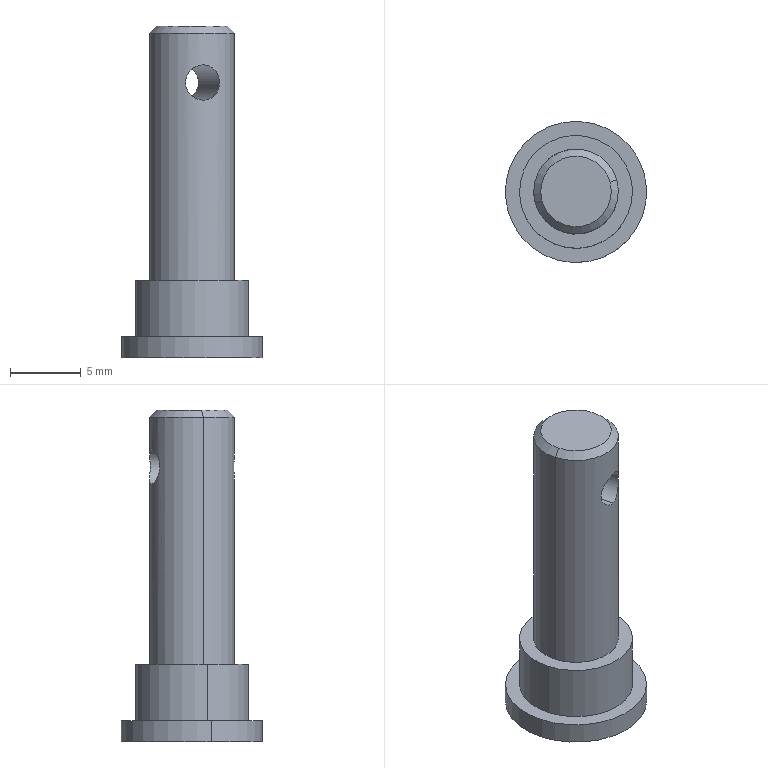Part | SolidWorks | features BaseBody 1 | 1 solid | 14 faces | box 10 x 10 x 23.5 mm | volume 796.786 mm3 | cylinder 8 | plane 4 | cone 2 | commonest cylinder face diameters 2.5 x2 6 x2 8 x2 10 x2
STEP:
#1=CARTESIAN_POINT('',(437.007,50.123,99.45));
#2=VERTEX_POINT('',#1);
#3=CARTESIAN_POINT('',(437.007,50.123,101.95));
#4=VERTEX_POINT('',#3);
#5=CARTESIAN_POINT('',(437.007,50.123,99.45));
#6=CARTESIAN_POINT('',(437.165,50.167,99.45));
#7=CARTESIAN_POINT('',(437.329,50.199,99.483));
#8=CARTESIAN_POINT('',(437.633,50.233,99.61));
#9=CARTESIAN_POINT('',(437.774,50.237,99.702));
#10=CARTESIAN_POINT('',(437.954,50.233,99.874));
#11=CARTESIAN_POINT('',(438.008,50.23,99.937));
#12=CARTESIAN_POINT('',(438.104,50.223,100.071));
#13=CARTESIAN_POINT('',(438.146,50.218,100.144));
#14=CARTESIAN_POINT('',(438.214,50.21,100.294));
#15=CARTESIAN_POINT('',(438.239,50.206,100.372));
#16=CARTESIAN_POINT('',(438.275,50.201,100.533));
#17=CARTESIAN_POINT('',(438.284,50.2,100.617));
#18=CARTESIAN_POINT('',(438.284,50.2,100.864));
#19=CARTESIAN_POINT('',(438.247,50.206,101.03));
#20=CARTESIAN_POINT('',(438.112,50.222,101.332));
#21=CARTESIAN_POINT('',(438.014,50.232,101.469));
#22=CARTESIAN_POINT('',(437.774,50.237,101.698));
#23=CARTESIAN_POINT('',(437.635,50.234,101.79));
#24=CARTESIAN_POINT('',(437.328,50.199,101.917));
#25=CARTESIAN_POINT('',(437.168,50.168,101.95));
#26=CARTESIAN_POINT('',(437.007,50.123,101.95));
#27=B_SPLINE_CURVE_WITH_KNOTS('',3,(#5,#6,#7,#8,#9,#10,#11,#12,#13,#14,#15,#16,#17,#18,#19,#20,#21,#22,#23,#24,#25,#26),.UNSPECIFIED.,.F.,.F.,(4,2,2,2,2,2,2,2,2,2,4),(0.003954,0.004448,0.004941,0.005188,0.005435,0.005682,0.005929,0.006423,0.006917,0.00741,0.007904),.UNSPECIFIED.);
#28=EDGE_CURVE('',#2,#4,#27,.T.);
#29=ORIENTED_EDGE('',*,*,#28,.F.);
#30=CARTESIAN_POINT('',(438.637,44.348,99.45));
#31=VERTEX_POINT('',#30);
#32=CARTESIAN_POINT('',(436.463,52.047,99.45));
#33=DIRECTION('',(0.2716,-0.9624,0.));
#34=VECTOR('',#33,1000.);
#35=LINE('',#32,#34);
#36=EDGE_CURVE('',#2,#31,#35,.T.);
#37=ORIENTED_EDGE('',*,*,#36,.T.);
#38=CARTESIAN_POINT('',(438.637,44.348,101.95));
#39=VERTEX_POINT('',#38);
#40=CARTESIAN_POINT('',(438.637,44.348,101.95));
#41=CARTESIAN_POINT('',(438.717,44.371,101.95));
#42=CARTESIAN_POINT('',(438.795,44.397,101.942));
#43=CARTESIAN_POINT('',(438.946,44.453,101.909));
#44=CARTESIAN_POINT('',(439.021,44.484,101.885));
#45=CARTESIAN_POINT('',(439.229,44.581,101.79));
#46=CARTESIAN_POINT('',(439.352,44.652,101.697));
#47=CARTESIAN_POINT('',(439.552,44.782,101.469));
#48=CARTESIAN_POINT('',(439.631,44.841,101.332));
#49=CARTESIAN_POINT('',(439.737,44.926,101.032));
#50=CARTESIAN_POINT('',(439.765,44.95,100.866));
#51=CARTESIAN_POINT('',(439.765,44.95,100.618));
#52=CARTESIAN_POINT('',(439.758,44.944,100.534));
#53=CARTESIAN_POINT('',(439.731,44.922,100.373));
#54=CARTESIAN_POINT('',(439.711,44.905,100.294));
#55=CARTESIAN_POINT('',(439.63,44.841,100.066));
#56=CARTESIAN_POINT('',(439.551,44.781,99.93));
#57=CARTESIAN_POINT('',(439.35,44.651,99.702));
#58=CARTESIAN_POINT('',(439.227,44.581,99.609));
#59=CARTESIAN_POINT('',(438.951,44.452,99.484));
#60=CARTESIAN_POINT('',(438.795,44.393,99.45));
#61=CARTESIAN_POINT('',(438.637,44.348,99.45));
#62=B_SPLINE_CURVE_WITH_KNOTS('',3,(#40,#41,#42,#43,#44,#45,#46,#47,#48,#49,#50,#51,#52,#53,#54,#55,#56,#57,#58,#59,#60,#61),.UNSPECIFIED.,.F.,.F.,(4,2,2,2,2,2,2,2,2,2,4),(0.,0.0002471,0.0004942,0.0009884,0.001483,0.001977,0.002224,0.002471,0.002965,0.003459,0.003954),.UNSPECIFIED.);
#63=EDGE_CURVE('',#39,#31,#62,.T.);
#64=ORIENTED_EDGE('',*,*,#63,.F.);
#65=CARTESIAN_POINT('',(436.463,52.047,101.95));
#66=DIRECTION('',(0.2716,-0.9624,0.));
#67=VECTOR('',#66,1000.);
#68=LINE('',#65,#67);
#69=EDGE_CURVE('',#4,#39,#68,.T.);
#70=ORIENTED_EDGE('',*,*,#69,.F.);
#71=EDGE_LOOP('',(#29,#37,#64,#70));
#72=FACE_OUTER_BOUND('',#71,.T.);
#73=CARTESIAN_POINT('',(436.463,52.047,100.7));
#74=DIRECTION('',(0.2716,-0.9624,0.));
#75=DIRECTION('',(0.,0.,1.));
#76=AXIS2_PLACEMENT_3D('',#73,#74,#75);
#77=CYLINDRICAL_SURFACE('',#76,1.25);
#78=ADVANCED_FACE('',(#72),#77,.F.);
#79=CARTESIAN_POINT('',(435.416,46.556,104.7));
#80=VERTEX_POINT('',#79);
#81=CARTESIAN_POINT('',(440.228,47.915,104.7));
#82=VERTEX_POINT('',#81);
#83=CARTESIAN_POINT('',(437.822,47.235,104.7));
#84=DIRECTION('',(0.,0.,1.));
#85=DIRECTION('',(-0.9624,-0.2716,0.));
#86=AXIS2_PLACEMENT_3D('',#83,#84,#85);
#87=CIRCLE('',#86,2.5);
#88=EDGE_CURVE('',#80,#82,#87,.T.);
#89=ORIENTED_EDGE('',*,*,#88,.F.);
#90=CARTESIAN_POINT('',(434.934,46.421,104.2));
#91=VERTEX_POINT('',#90);
#92=CARTESIAN_POINT('',(435.416,46.556,104.7));
#93=DIRECTION('',(-0.6805,-0.1921,-0.7071));
#94=VECTOR('',#93,1000.);
#95=LINE('',#92,#94);
#96=EDGE_CURVE('',#80,#91,#95,.T.);
#97=ORIENTED_EDGE('',*,*,#96,.T.);
#98=CARTESIAN_POINT('',(440.709,48.05,104.2));
#99=VERTEX_POINT('',#98);
#100=CARTESIAN_POINT('',(437.822,47.235,104.2));
#101=DIRECTION('',(0.,0.,-1.));
#102=DIRECTION('',(-0.9624,-0.2716,0.));
#103=AXIS2_PLACEMENT_3D('',#100,#101,#102);
#104=CIRCLE('',#103,3.);
#105=EDGE_CURVE('',#99,#91,#104,.T.);
#106=ORIENTED_EDGE('',*,*,#105,.F.);
#107=CARTESIAN_POINT('',(440.228,47.915,104.7));
#108=DIRECTION('',(0.6805,0.1921,-0.7071));
#109=VECTOR('',#108,1000.);
#110=LINE('',#107,#109);
#111=EDGE_CURVE('',#82,#99,#110,.T.);
#112=ORIENTED_EDGE('',*,*,#111,.F.);
#113=EDGE_LOOP('',(#89,#97,#106,#112));
#114=FACE_OUTER_BOUND('',#113,.T.);
#115=CARTESIAN_POINT('',(437.822,47.235,104.7));
#116=DIRECTION('',(0.,0.,-1.));
#117=DIRECTION('',(0.9624,0.2716,0.));
#118=AXIS2_PLACEMENT_3D('',#115,#116,#117);
#119=CONICAL_SURFACE('',#118,2.5,0.7854);
#120=ADVANCED_FACE('',(#114),#119,.T.);
#121=ORIENTED_EDGE('',*,*,#63,.T.);
#122=CARTESIAN_POINT('',(438.637,44.348,99.45));
#123=CARTESIAN_POINT('',(438.478,44.304,99.45));
#124=CARTESIAN_POINT('',(438.315,44.272,99.483));
#125=CARTESIAN_POINT('',(438.01,44.237,99.61));
#126=CARTESIAN_POINT('',(437.869,44.233,99.702));
#127=CARTESIAN_POINT('',(437.689,44.238,99.874));
#128=CARTESIAN_POINT('',(437.635,44.241,99.937));
#129=CARTESIAN_POINT('',(437.539,44.248,100.071));
#130=CARTESIAN_POINT('',(437.497,44.253,100.144));
#131=CARTESIAN_POINT('',(437.43,44.261,100.294));
#132=CARTESIAN_POINT('',(437.404,44.265,100.372));
#133=CARTESIAN_POINT('',(437.369,44.27,100.533));
#134=CARTESIAN_POINT('',(437.359,44.271,100.617));
#135=CARTESIAN_POINT('',(437.359,44.271,100.864));
#136=CARTESIAN_POINT('',(437.396,44.265,101.03));
#137=CARTESIAN_POINT('',(437.531,44.249,101.332));
#138=CARTESIAN_POINT('',(437.629,44.239,101.469));
#139=CARTESIAN_POINT('',(437.869,44.233,101.698));
#140=CARTESIAN_POINT('',(438.009,44.237,101.79));
#141=CARTESIAN_POINT('',(438.315,44.272,101.917));
#142=CARTESIAN_POINT('',(438.476,44.303,101.95));
#143=CARTESIAN_POINT('',(438.637,44.348,101.95));
#144=B_SPLINE_CURVE_WITH_KNOTS('',3,(#122,#123,#124,#125,#126,#127,#128,#129,#130,#131,#132,#133,#134,#135,#136,#137,#138,#139,#140,#141,#142,#143),.UNSPECIFIED.,.F.,.F.,(4,2,2,2,2,2,2,2,2,2,4),(0.003954,0.004448,0.004941,0.005188,0.005435,0.005682,0.005929,0.006423,0.006917,0.00741,0.007904),.UNSPECIFIED.);
#145=EDGE_CURVE('',#31,#39,#144,.T.);
#146=ORIENTED_EDGE('',*,*,#145,.T.);
#147=EDGE_LOOP('',(#121,#146));
#148=FACE_BOUND('',#147,.T.);
#149=ORIENTED_EDGE('',*,*,#105,.T.);
#150=CARTESIAN_POINT('',(434.934,46.421,86.7));
#151=VERTEX_POINT('',#150);
#152=CARTESIAN_POINT('',(434.934,46.421,104.7));
#153=DIRECTION('',(0.,0.,-1.));
#154=VECTOR('',#153,1000.);
#155=LINE('',#152,#154);
#156=EDGE_CURVE('',#91,#151,#155,.T.);
#157=ORIENTED_EDGE('',*,*,#156,.T.);
#158=CARTESIAN_POINT('',(440.709,48.05,86.7));
#159=VERTEX_POINT('',#158);
#160=CARTESIAN_POINT('',(437.822,47.235,86.7));
#161=DIRECTION('',(0.,0.,1.));
#162=DIRECTION('',(-0.9624,-0.2716,0.));
#163=AXIS2_PLACEMENT_3D('',#160,#161,#162);
#164=CIRCLE('',#163,3.);
#165=EDGE_CURVE('',#151,#159,#164,.T.);
#166=ORIENTED_EDGE('',*,*,#165,.T.);
#167=CARTESIAN_POINT('',(440.709,48.05,104.7));
#168=DIRECTION('',(0.,0.,-1.));
#169=VECTOR('',#168,1000.);
#170=LINE('',#167,#169);
#171=EDGE_CURVE('',#99,#159,#170,.T.);
#172=ORIENTED_EDGE('',*,*,#171,.F.);
#173=EDGE_LOOP('',(#149,#157,#166,#172));
#174=FACE_OUTER_BOUND('',#173,.T.);
#175=CARTESIAN_POINT('',(437.822,47.235,104.7));
#176=DIRECTION('',(0.,0.,-1.));
#177=DIRECTION('',(0.9624,0.2716,0.));
#178=AXIS2_PLACEMENT_3D('',#175,#176,#177);
#179=CYLINDRICAL_SURFACE('',#178,3.);
#180=ADVANCED_FACE('',(#148,#174),#179,.T.);
#181=CARTESIAN_POINT('',(433.972,46.149,86.7));
#182=VERTEX_POINT('',#181);
#183=CARTESIAN_POINT('',(441.671,48.322,86.7));
#184=VERTEX_POINT('',#183);
#185=CARTESIAN_POINT('',(437.822,47.235,86.7));
#186=DIRECTION('',(0.,0.,1.));
#187=DIRECTION('',(-0.9624,-0.2716,0.));
#188=AXIS2_PLACEMENT_3D('',#185,#186,#187);
#189=CIRCLE('',#188,4.);
#190=EDGE_CURVE('',#182,#184,#189,.T.);
#191=ORIENTED_EDGE('',*,*,#190,.F.);
#192=CARTESIAN_POINT('',(433.972,46.149,82.7));
#193=VERTEX_POINT('',#192);
#194=CARTESIAN_POINT('',(433.972,46.149,86.7));
#195=DIRECTION('',(0.,0.,-1.));
#196=VECTOR('',#195,1000.);
#197=LINE('',#194,#196);
#198=EDGE_CURVE('',#182,#193,#197,.T.);
#199=ORIENTED_EDGE('',*,*,#198,.T.);
#200=CARTESIAN_POINT('',(441.671,48.322,82.7));
#201=VERTEX_POINT('',#200);
#202=CARTESIAN_POINT('',(437.822,47.235,82.7));
#203=DIRECTION('',(0.,0.,1.));
#204=DIRECTION('',(-0.9624,-0.2716,0.));
#205=AXIS2_PLACEMENT_3D('',#202,#203,#204);
#206=CIRCLE('',#205,4.);
#207=EDGE_CURVE('',#193,#201,#206,.T.);
#208=ORIENTED_EDGE('',*,*,#207,.T.);
#209=CARTESIAN_POINT('',(441.671,48.322,86.7));
#210=DIRECTION('',(0.,0.,-1.));
#211=VECTOR('',#210,1000.);
#212=LINE('',#209,#211);
#213=EDGE_CURVE('',#184,#201,#212,.T.);
#214=ORIENTED_EDGE('',*,*,#213,.F.);
#215=EDGE_LOOP('',(#191,#199,#208,#214));
#216=FACE_OUTER_BOUND('',#215,.T.);
#217=CARTESIAN_POINT('',(437.822,47.235,86.7));
#218=DIRECTION('',(0.,0.,-1.));
#219=DIRECTION('',(0.9624,0.2716,0.));
#220=AXIS2_PLACEMENT_3D('',#217,#218,#219);
#221=CYLINDRICAL_SURFACE('',#220,4.);
#222=ADVANCED_FACE('',(#216),#221,.T.);
#223=CARTESIAN_POINT('',(433.01,45.877,82.7));
#224=VERTEX_POINT('',#223);
#225=CARTESIAN_POINT('',(442.634,48.594,82.7));
#226=VERTEX_POINT('',#225);
#227=CARTESIAN_POINT('',(437.822,47.235,82.7));
#228=DIRECTION('',(0.,0.,1.));
#229=DIRECTION('',(-0.9624,-0.2716,0.));
#230=AXIS2_PLACEMENT_3D('',#227,#228,#229);
#231=CIRCLE('',#230,5.);
#232=EDGE_CURVE('',#224,#226,#231,.T.);
#233=ORIENTED_EDGE('',*,*,#232,.F.);
#234=CARTESIAN_POINT('',(433.01,45.877,81.2));
#235=VERTEX_POINT('',#234);
#236=CARTESIAN_POINT('',(433.01,45.877,82.7));
#237=DIRECTION('',(0.,0.,-1.));
#238=VECTOR('',#237,1000.);
#239=LINE('',#236,#238);
#240=EDGE_CURVE('',#224,#235,#239,.T.);
#241=ORIENTED_EDGE('',*,*,#240,.T.);
#242=CARTESIAN_POINT('',(442.634,48.594,81.2));
#243=VERTEX_POINT('',#242);
#244=CARTESIAN_POINT('',(437.822,47.235,81.2));
#245=DIRECTION('',(0.,0.,1.));
#246=DIRECTION('',(-0.9624,-0.2716,0.));
#247=AXIS2_PLACEMENT_3D('',#244,#245,#246);
#248=CIRCLE('',#247,5.);
#249=EDGE_CURVE('',#235,#243,#248,.T.);
#250=ORIENTED_EDGE('',*,*,#249,.T.);
#251=CARTESIAN_POINT('',(442.634,48.594,82.7));
#252=DIRECTION('',(0.,0.,-1.));
#253=VECTOR('',#252,1000.);
#254=LINE('',#251,#253);
#255=EDGE_CURVE('',#226,#243,#254,.T.);
#256=ORIENTED_EDGE('',*,*,#255,.F.);
#257=EDGE_LOOP('',(#233,#241,#250,#256));
#258=FACE_OUTER_BOUND('',#257,.T.);
#259=CARTESIAN_POINT('',(437.822,47.235,82.7));
#260=DIRECTION('',(0.,0.,-1.));
#261=DIRECTION('',(0.9624,0.2716,0.));
#262=AXIS2_PLACEMENT_3D('',#259,#260,#261);
#263=CYLINDRICAL_SURFACE('',#262,5.);
#264=ADVANCED_FACE('',(#258),#263,.T.);
#265=CARTESIAN_POINT('',(437.822,47.235,86.7));
#266=DIRECTION('',(0.,0.,1.));
#267=DIRECTION('',(-0.9624,-0.2716,0.));
#268=AXIS2_PLACEMENT_3D('',#265,#266,#267);
#269=CIRCLE('',#268,4.);
#270=EDGE_CURVE('',#184,#182,#269,.T.);
#271=ORIENTED_EDGE('',*,*,#270,.T.);
#272=ORIENTED_EDGE('',*,*,#190,.T.);
#273=EDGE_LOOP('',(#271,#272));
#274=FACE_OUTER_BOUND('',#273,.T.);
#275=CARTESIAN_POINT('',(437.822,47.235,86.7));
#276=DIRECTION('',(0.,0.,1.));
#277=DIRECTION('',(-0.9624,-0.2716,0.));
#278=AXIS2_PLACEMENT_3D('',#275,#276,#277);
#279=CIRCLE('',#278,3.);
#280=EDGE_CURVE('',#159,#151,#279,.T.);
#281=ORIENTED_EDGE('',*,*,#280,.F.);
#282=ORIENTED_EDGE('',*,*,#165,.F.);
#283=EDGE_LOOP('',(#281,#282));
#284=FACE_BOUND('',#283,.T.);
#285=CARTESIAN_POINT('',(437.822,47.235,86.7));
#286=DIRECTION('',(0.,0.,1.));
#287=DIRECTION('',(-0.9624,-0.2716,0.));
#288=AXIS2_PLACEMENT_3D('',#285,#286,#287);
#289=PLANE('',#288);
#290=ADVANCED_FACE('',(#274,#284),#289,.T.);
#291=CARTESIAN_POINT('',(437.822,47.235,82.7));
#292=DIRECTION('',(0.,0.,1.));
#293=DIRECTION('',(-0.9624,-0.2716,0.));
#294=AXIS2_PLACEMENT_3D('',#291,#292,#293);
#295=CIRCLE('',#294,5.);
#296=EDGE_CURVE('',#226,#224,#295,.T.);
#297=ORIENTED_EDGE('',*,*,#296,.T.);
#298=ORIENTED_EDGE('',*,*,#232,.T.);
#299=EDGE_LOOP('',(#297,#298));
#300=FACE_OUTER_BOUND('',#299,.T.);
#301=CARTESIAN_POINT('',(437.822,47.235,82.7));
#302=DIRECTION('',(0.,0.,1.));
#303=DIRECTION('',(-0.9624,-0.2716,0.));
#304=AXIS2_PLACEMENT_3D('',#301,#302,#303);
#305=CIRCLE('',#304,4.);
#306=EDGE_CURVE('',#201,#193,#305,.T.);
#307=ORIENTED_EDGE('',*,*,#306,.F.);
#308=ORIENTED_EDGE('',*,*,#207,.F.);
#309=EDGE_LOOP('',(#307,#308));
#310=FACE_BOUND('',#309,.T.);
#311=CARTESIAN_POINT('',(437.822,47.235,82.7));
#312=DIRECTION('',(0.,0.,1.));
#313=DIRECTION('',(-0.9624,-0.2716,0.));
#314=AXIS2_PLACEMENT_3D('',#311,#312,#313);
#315=PLANE('',#314);
#316=ADVANCED_FACE('',(#300,#310),#315,.T.);
#317=ORIENTED_EDGE('',*,*,#240,.F.);
#318=ORIENTED_EDGE('',*,*,#296,.F.);
#319=ORIENTED_EDGE('',*,*,#255,.T.);
#320=CARTESIAN_POINT('',(437.822,47.235,81.2));
#321=DIRECTION('',(0.,0.,1.));
#322=DIRECTION('',(-0.9624,-0.2716,0.));
#323=AXIS2_PLACEMENT_3D('',#320,#321,#322);
#324=CIRCLE('',#323,5.);
#325=EDGE_CURVE('',#243,#235,#324,.T.);
#326=ORIENTED_EDGE('',*,*,#325,.T.);
#327=EDGE_LOOP('',(#317,#318,#319,#326));
#328=FACE_OUTER_BOUND('',#327,.T.);
#329=CARTESIAN_POINT('',(437.822,47.235,82.7));
#330=DIRECTION('',(0.,0.,-1.));
#331=DIRECTION('',(0.9624,0.2716,0.));
#332=AXIS2_PLACEMENT_3D('',#329,#330,#331);
#333=CYLINDRICAL_SURFACE('',#332,5.);
#334=ADVANCED_FACE('',(#328),#333,.T.);
#335=ORIENTED_EDGE('',*,*,#325,.F.);
#336=ORIENTED_EDGE('',*,*,#249,.F.);
#337=EDGE_LOOP('',(#335,#336));
#338=FACE_OUTER_BOUND('',#337,.T.);
#339=CARTESIAN_POINT('',(437.822,47.235,81.2));
#340=DIRECTION('',(0.,0.,1.));
#341=DIRECTION('',(-0.9624,-0.2716,0.));
#342=AXIS2_PLACEMENT_3D('',#339,#340,#341);
#343=PLANE('',#342);
#344=ADVANCED_FACE('',(#338),#343,.F.);
#345=ORIENTED_EDGE('',*,*,#198,.F.);
#346=ORIENTED_EDGE('',*,*,#270,.F.);
#347=ORIENTED_EDGE('',*,*,#213,.T.);
#348=ORIENTED_EDGE('',*,*,#306,.T.);
#349=EDGE_LOOP('',(#345,#346,#347,#348));
#350=FACE_OUTER_BOUND('',#349,.T.);
#351=CARTESIAN_POINT('',(437.822,47.235,86.7));
#352=DIRECTION('',(0.,0.,-1.));
#353=DIRECTION('',(0.9624,0.2716,0.));
#354=AXIS2_PLACEMENT_3D('',#351,#352,#353);
#355=CYLINDRICAL_SURFACE('',#354,4.);
#356=ADVANCED_FACE('',(#350),#355,.T.);
#357=ORIENTED_EDGE('',*,*,#156,.F.);
#358=CARTESIAN_POINT('',(437.822,47.235,104.2));
#359=DIRECTION('',(0.,0.,-1.));
#360=DIRECTION('',(-0.9624,-0.2716,0.));
#361=AXIS2_PLACEMENT_3D('',#358,#359,#360);
#362=CIRCLE('',#361,3.);
#363=EDGE_CURVE('',#91,#99,#362,.T.);
#364=ORIENTED_EDGE('',*,*,#363,.T.);
#365=ORIENTED_EDGE('',*,*,#171,.T.);
#366=ORIENTED_EDGE('',*,*,#280,.T.);
#367=EDGE_LOOP('',(#357,#364,#365,#366));
#368=FACE_OUTER_BOUND('',#367,.T.);
#369=CARTESIAN_POINT('',(437.007,50.123,101.95));
#370=CARTESIAN_POINT('',(436.926,50.1,101.95));
#371=CARTESIAN_POINT('',(436.848,50.074,101.942));
#372=CARTESIAN_POINT('',(436.697,50.018,101.909));
#373=CARTESIAN_POINT('',(436.623,49.986,101.885));
#374=CARTESIAN_POINT('',(436.415,49.889,101.79));
#375=CARTESIAN_POINT('',(436.292,49.819,101.697));
#376=CARTESIAN_POINT('',(436.092,49.689,101.469));
#377=CARTESIAN_POINT('',(436.012,49.629,101.332));
#378=CARTESIAN_POINT('',(435.906,49.545,101.032));
#379=CARTESIAN_POINT('',(435.878,49.521,100.866));
#380=CARTESIAN_POINT('',(435.878,49.521,100.618));
#381=CARTESIAN_POINT('',(435.885,49.527,100.534));
#382=CARTESIAN_POINT('',(435.912,49.549,100.373));
#383=CARTESIAN_POINT('',(435.932,49.566,100.294));
#384=CARTESIAN_POINT('',(436.013,49.63,100.066));
#385=CARTESIAN_POINT('',(436.092,49.69,99.93));
#386=CARTESIAN_POINT('',(436.293,49.82,99.702));
#387=CARTESIAN_POINT('',(436.416,49.89,99.609));
#388=CARTESIAN_POINT('',(436.692,50.019,99.484));
#389=CARTESIAN_POINT('',(436.848,50.078,99.45));
#390=CARTESIAN_POINT('',(437.007,50.123,99.45));
#391=B_SPLINE_CURVE_WITH_KNOTS('',3,(#369,#370,#371,#372,#373,#374,#375,#376,#377,#378,#379,#380,#381,#382,#383,#384,#385,#386,#387,#388,#389,#390),.UNSPECIFIED.,.F.,.F.,(4,2,2,2,2,2,2,2,2,2,4),(0.,0.0002471,0.0004942,0.0009884,0.001483,0.001977,0.002224,0.002471,0.002965,0.003459,0.003954),.UNSPECIFIED.);
#392=EDGE_CURVE('',#4,#2,#391,.T.);
#393=ORIENTED_EDGE('',*,*,#392,.T.);
#394=ORIENTED_EDGE('',*,*,#28,.T.);
#395=EDGE_LOOP('',(#393,#394));
#396=FACE_BOUND('',#395,.T.);
#397=CARTESIAN_POINT('',(437.822,47.235,104.7));
#398=DIRECTION('',(0.,0.,-1.));
#399=DIRECTION('',(0.9624,0.2716,0.));
#400=AXIS2_PLACEMENT_3D('',#397,#398,#399);
#401=CYLINDRICAL_SURFACE('',#400,3.);
#402=ADVANCED_FACE('',(#368,#396),#401,.T.);
#403=CARTESIAN_POINT('',(437.822,47.235,104.7));
#404=DIRECTION('',(0.,0.,1.));
#405=DIRECTION('',(-0.9624,-0.2716,0.));
#406=AXIS2_PLACEMENT_3D('',#403,#404,#405);
#407=CIRCLE('',#406,2.5);
#408=EDGE_CURVE('',#82,#80,#407,.T.);
#409=ORIENTED_EDGE('',*,*,#408,.T.);
#410=ORIENTED_EDGE('',*,*,#88,.T.);
#411=EDGE_LOOP('',(#409,#410));
#412=FACE_OUTER_BOUND('',#411,.T.);
#413=CARTESIAN_POINT('',(437.822,47.235,104.7));
#414=DIRECTION('',(0.,0.,1.));
#415=DIRECTION('',(-0.9624,-0.2716,0.));
#416=AXIS2_PLACEMENT_3D('',#413,#414,#415);
#417=PLANE('',#416);
#418=ADVANCED_FACE('',(#412),#417,.T.);
#419=ORIENTED_EDGE('',*,*,#96,.F.);
#420=ORIENTED_EDGE('',*,*,#408,.F.);
#421=ORIENTED_EDGE('',*,*,#111,.T.);
#422=ORIENTED_EDGE('',*,*,#363,.F.);
#423=EDGE_LOOP('',(#419,#420,#421,#422));
#424=FACE_OUTER_BOUND('',#423,.T.);
#425=CARTESIAN_POINT('',(437.822,47.235,104.7));
#426=DIRECTION('',(0.,0.,-1.));
#427=DIRECTION('',(0.9624,0.2716,0.));
#428=AXIS2_PLACEMENT_3D('',#425,#426,#427);
#429=CONICAL_SURFACE('',#428,2.5,0.7854);
#430=ADVANCED_FACE('',(#424),#429,.T.);
#431=ORIENTED_EDGE('',*,*,#36,.F.);
#432=ORIENTED_EDGE('',*,*,#392,.F.);
#433=ORIENTED_EDGE('',*,*,#69,.T.);
#434=ORIENTED_EDGE('',*,*,#145,.F.);
#435=EDGE_LOOP('',(#431,#432,#433,#434));
#436=FACE_OUTER_BOUND('',#435,.T.);
#437=CARTESIAN_POINT('',(436.463,52.047,100.7));
#438=DIRECTION('',(0.2716,-0.9624,0.));
#439=DIRECTION('',(0.,0.,1.));
#440=AXIS2_PLACEMENT_3D('',#437,#438,#439);
#441=CYLINDRICAL_SURFACE('',#440,1.25);
#442=ADVANCED_FACE('',(#436),#441,.F.);
#443=CLOSED_SHELL('',(#78,#120,#180,#222,#264,#290,#316,#334,#344,#356,#402,#418,#430,#442));
#444=MANIFOLD_SOLID_BREP('',#443);
#445=CARTESIAN_POINT('',(0.,0.,0.));
#446=DIRECTION('',(0.,0.,1.));
#447=DIRECTION('',(1.,0.,0.));
#448=AXIS2_PLACEMENT_3D('',#445,#446,#447);
#449=(LENGTH_UNIT()NAMED_UNIT(*)SI_UNIT(.MILLI.,.METRE.));
#450=UNCERTAINTY_MEASURE_WITH_UNIT(LENGTH_MEASURE(0.00001),#449,'','');
#451=(NAMED_UNIT(*)PLANE_ANGLE_UNIT()SI_UNIT($,.RADIAN.));
#452=(NAMED_UNIT(*)SI_UNIT($,.STERADIAN.)SOLID_ANGLE_UNIT());
#453=(GEOMETRIC_REPRESENTATION_CONTEXT(3)GLOBAL_UNCERTAINTY_ASSIGNED_CONTEXT((#450))GLOBAL_UNIT_ASSIGNED_CONTEXT((#449,#451,#452))REPRESENTATION_CONTEXT('',''));
#454=ADVANCED_BREP_SHAPE_REPRESENTATION('',(#444,#448),#453);